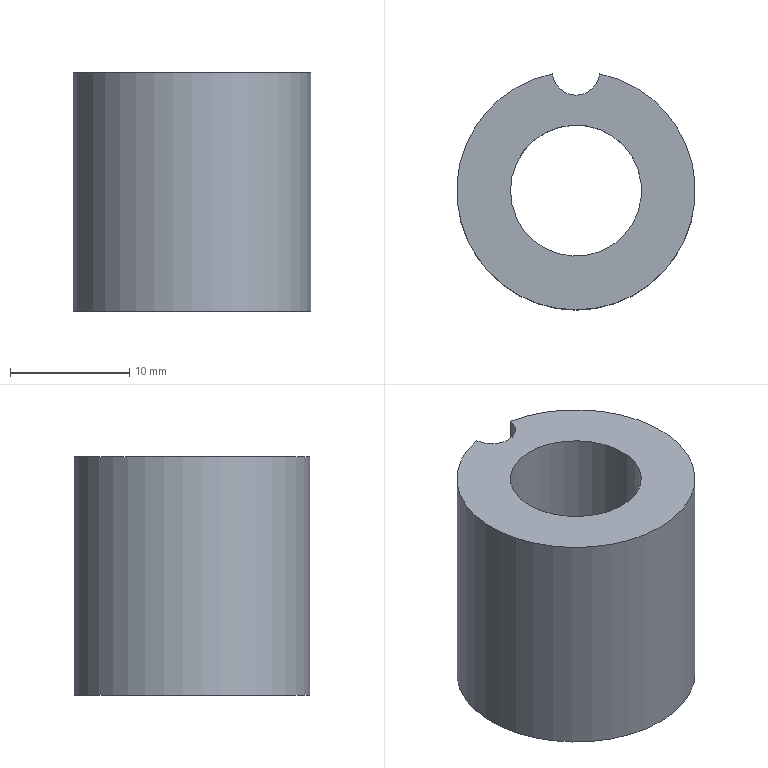Part | NX | features solid 2 | 1 solid | 7 faces | box 20 x 19.8 x 20 mm | volume 3906 mm3 | cylinder 4 | plane 3 | commonest cylinder face diameters 4 x1 11 x1 12.6 x1 20 x1
STEP:
#1=CARTESIAN_POINT('',(1589.99,141.792,7.));
#2=VERTEX_POINT('',#1);
#3=CARTESIAN_POINT('',(1589.99,141.792,27.));
#4=VERTEX_POINT('',#3);
#5=CARTESIAN_POINT('',(1589.99,141.792,14.5));
#6=DIRECTION('',(0.,0.,1.));
#7=VECTOR('',#6,1000.);
#8=LINE('',#5,#7);
#9=EDGE_CURVE('',#2,#4,#8,.T.);
#10=ORIENTED_EDGE('',*,*,#9,.T.);
#11=CARTESIAN_POINT('',(1586.01,141.792,27.));
#12=VERTEX_POINT('',#11);
#13=CARTESIAN_POINT('',(1588.,131.992,27.));
#14=DIRECTION('',(0.,0.,-1.));
#15=DIRECTION('',(0.,1.,0.));
#16=AXIS2_PLACEMENT_3D('',#13,#14,#15);
#17=CIRCLE('',#16,10.);
#18=EDGE_CURVE('',#4,#12,#17,.T.);
#19=ORIENTED_EDGE('',*,*,#18,.T.);
#20=CARTESIAN_POINT('',(1586.01,141.792,7.));
#21=VERTEX_POINT('',#20);
#22=CARTESIAN_POINT('',(1586.01,141.792,14.5));
#23=DIRECTION('',(0.,0.,1.));
#24=VECTOR('',#23,1000.);
#25=LINE('',#22,#24);
#26=EDGE_CURVE('',#12,#21,#25,.F.);
#27=ORIENTED_EDGE('',*,*,#26,.T.);
#28=CARTESIAN_POINT('',(1588.,131.992,7.));
#29=DIRECTION('',(0.,0.,1.));
#30=DIRECTION('',(1.,0.,0.));
#31=AXIS2_PLACEMENT_3D('',#28,#29,#30);
#32=CIRCLE('',#31,10.);
#33=EDGE_CURVE('',#2,#21,#32,.F.);
#34=ORIENTED_EDGE('',*,*,#33,.F.);
#35=EDGE_LOOP('',(#10,#19,#27,#34));
#36=FACE_BOUND('',#35,.T.);
#37=CARTESIAN_POINT('',(1588.,131.992,2.));
#38=DIRECTION('',(0.,0.,1.));
#39=DIRECTION('',(0.,1.,0.));
#40=AXIS2_PLACEMENT_3D('',#37,#38,#39);
#41=CYLINDRICAL_SURFACE('',#40,10.);
#42=ADVANCED_FACE('',(#36),#41,.T.);
#43=CARTESIAN_POINT('',(1594.3,131.992,7.));
#44=VERTEX_POINT('',#43);
#45=CARTESIAN_POINT('',(1588.,131.992,7.));
#46=DIRECTION('',(0.,0.,1.));
#47=DIRECTION('',(1.,0.,0.));
#48=AXIS2_PLACEMENT_3D('',#45,#46,#47);
#49=CIRCLE('',#48,6.3);
#50=EDGE_CURVE('',#44,#44,#49,.F.);
#51=ORIENTED_EDGE('',*,*,#50,.F.);
#52=EDGE_LOOP('',(#51));
#53=FACE_BOUND('',#52,.T.);
#54=ORIENTED_EDGE('',*,*,#33,.T.);
#55=CARTESIAN_POINT('',(1588.,141.992,7.));
#56=DIRECTION('',(0.,0.,1.));
#57=DIRECTION('',(1.,0.,0.));
#58=AXIS2_PLACEMENT_3D('',#55,#56,#57);
#59=CIRCLE('',#58,2.);
#60=EDGE_CURVE('',#2,#21,#59,.F.);
#61=ORIENTED_EDGE('',*,*,#60,.F.);
#62=EDGE_LOOP('',(#54,#61));
#63=FACE_BOUND('',#62,.T.);
#64=CARTESIAN_POINT('',(1588.,131.992,7.));
#65=DIRECTION('',(0.,0.,1.));
#66=DIRECTION('',(0.,1.,0.));
#67=AXIS2_PLACEMENT_3D('',#64,#65,#66);
#68=PLANE('',#67);
#69=ADVANCED_FACE('',(#53,#63),#68,.F.);
#70=CARTESIAN_POINT('',(1582.5,131.992,27.));
#71=VERTEX_POINT('',#70);
#72=CARTESIAN_POINT('',(1588.,131.992,27.));
#73=DIRECTION('',(0.,0.,-1.));
#74=DIRECTION('',(-1.,0.,0.));
#75=AXIS2_PLACEMENT_3D('',#72,#73,#74);
#76=CIRCLE('',#75,5.5);
#77=EDGE_CURVE('',#71,#71,#76,.T.);
#78=ORIENTED_EDGE('',*,*,#77,.T.);
#79=EDGE_LOOP('',(#78));
#80=FACE_BOUND('',#79,.T.);
#81=CARTESIAN_POINT('',(1588.,141.992,27.));
#82=DIRECTION('',(0.,0.,-1.));
#83=DIRECTION('',(0.,1.,0.));
#84=AXIS2_PLACEMENT_3D('',#81,#82,#83);
#85=CIRCLE('',#84,2.);
#86=EDGE_CURVE('',#4,#12,#85,.T.);
#87=ORIENTED_EDGE('',*,*,#86,.T.);
#88=ORIENTED_EDGE('',*,*,#18,.F.);
#89=EDGE_LOOP('',(#87,#88));
#90=FACE_BOUND('',#89,.T.);
#91=CARTESIAN_POINT('',(1588.,131.992,27.));
#92=DIRECTION('',(0.,0.,1.));
#93=DIRECTION('',(0.,1.,0.));
#94=AXIS2_PLACEMENT_3D('',#91,#92,#93);
#95=PLANE('',#94);
#96=ADVANCED_FACE('',(#80,#90),#95,.T.);
#97=ORIENTED_EDGE('',*,*,#50,.T.);
#98=EDGE_LOOP('',(#97));
#99=FACE_BOUND('',#98,.T.);
#100=CARTESIAN_POINT('',(1588.,138.292,19.));
#101=VERTEX_POINT('',#100);
#102=CARTESIAN_POINT('',(1588.,131.992,19.));
#103=DIRECTION('',(0.,0.,-1.));
#104=DIRECTION('',(0.,1.,0.));
#105=AXIS2_PLACEMENT_3D('',#102,#103,#104);
#106=CIRCLE('',#105,6.3);
#107=EDGE_CURVE('',#101,#101,#106,.T.);
#108=ORIENTED_EDGE('',*,*,#107,.F.);
#109=EDGE_LOOP('',(#108));
#110=FACE_BOUND('',#109,.T.);
#111=CARTESIAN_POINT('',(1588.,131.992,2.));
#112=DIRECTION('',(0.,0.,1.));
#113=DIRECTION('',(0.,1.,0.));
#114=AXIS2_PLACEMENT_3D('',#111,#112,#113);
#115=CYLINDRICAL_SURFACE('',#114,6.3);
#116=ADVANCED_FACE('',(#99,#110),#115,.F.);
#117=CARTESIAN_POINT('',(1582.5,131.992,19.));
#118=VERTEX_POINT('',#117);
#119=CARTESIAN_POINT('',(1588.,131.992,19.));
#120=DIRECTION('',(0.,0.,-1.));
#121=DIRECTION('',(-1.,0.,0.));
#122=AXIS2_PLACEMENT_3D('',#119,#120,#121);
#123=CIRCLE('',#122,5.5);
#124=EDGE_CURVE('',#118,#118,#123,.T.);
#125=ORIENTED_EDGE('',*,*,#124,.F.);
#126=EDGE_LOOP('',(#125));
#127=FACE_BOUND('',#126,.T.);
#128=ORIENTED_EDGE('',*,*,#107,.T.);
#129=EDGE_LOOP('',(#128));
#130=FACE_BOUND('',#129,.T.);
#131=CARTESIAN_POINT('',(1588.,131.992,19.));
#132=DIRECTION('',(0.,0.,1.));
#133=DIRECTION('',(0.,1.,0.));
#134=AXIS2_PLACEMENT_3D('',#131,#132,#133);
#135=PLANE('',#134);
#136=ADVANCED_FACE('',(#127,#130),#135,.F.);
#137=ORIENTED_EDGE('',*,*,#9,.F.);
#138=ORIENTED_EDGE('',*,*,#60,.T.);
#139=ORIENTED_EDGE('',*,*,#26,.F.);
#140=ORIENTED_EDGE('',*,*,#86,.F.);
#141=EDGE_LOOP('',(#137,#138,#139,#140));
#142=FACE_BOUND('',#141,.T.);
#143=CARTESIAN_POINT('',(1588.,141.992,2.));
#144=DIRECTION('',(0.,0.,1.));
#145=DIRECTION('',(0.,1.,0.));
#146=AXIS2_PLACEMENT_3D('',#143,#144,#145);
#147=CYLINDRICAL_SURFACE('',#146,2.);
#148=ADVANCED_FACE('',(#142),#147,.F.);
#149=ORIENTED_EDGE('',*,*,#77,.F.);
#150=EDGE_LOOP('',(#149));
#151=FACE_BOUND('',#150,.T.);
#152=ORIENTED_EDGE('',*,*,#124,.T.);
#153=EDGE_LOOP('',(#152));
#154=FACE_BOUND('',#153,.T.);
#155=CARTESIAN_POINT('',(1588.,131.992,2.));
#156=DIRECTION('',(0.,0.,1.));
#157=DIRECTION('',(0.,1.,0.));
#158=AXIS2_PLACEMENT_3D('',#155,#156,#157);
#159=CYLINDRICAL_SURFACE('',#158,5.5);
#160=ADVANCED_FACE('',(#151,#154),#159,.F.);
#161=CLOSED_SHELL('',(#42,#69,#96,#116,#136,#148,#160));
#162=MANIFOLD_SOLID_BREP('',#161);
#163=(LENGTH_UNIT()NAMED_UNIT(*)SI_UNIT(.MILLI.,.METRE.));
#164=UNCERTAINTY_MEASURE_WITH_UNIT(LENGTH_MEASURE(0.00001),#163,'','');
#165=(NAMED_UNIT(*)PLANE_ANGLE_UNIT()SI_UNIT($,.RADIAN.));
#166=(NAMED_UNIT(*)SI_UNIT($,.STERADIAN.)SOLID_ANGLE_UNIT());
#167=(GEOMETRIC_REPRESENTATION_CONTEXT(3)GLOBAL_UNCERTAINTY_ASSIGNED_CONTEXT((#164))GLOBAL_UNIT_ASSIGNED_CONTEXT((#163,#165,#166))REPRESENTATION_CONTEXT('',''));
#168=ADVANCED_BREP_SHAPE_REPRESENTATION('',(#162),#167);